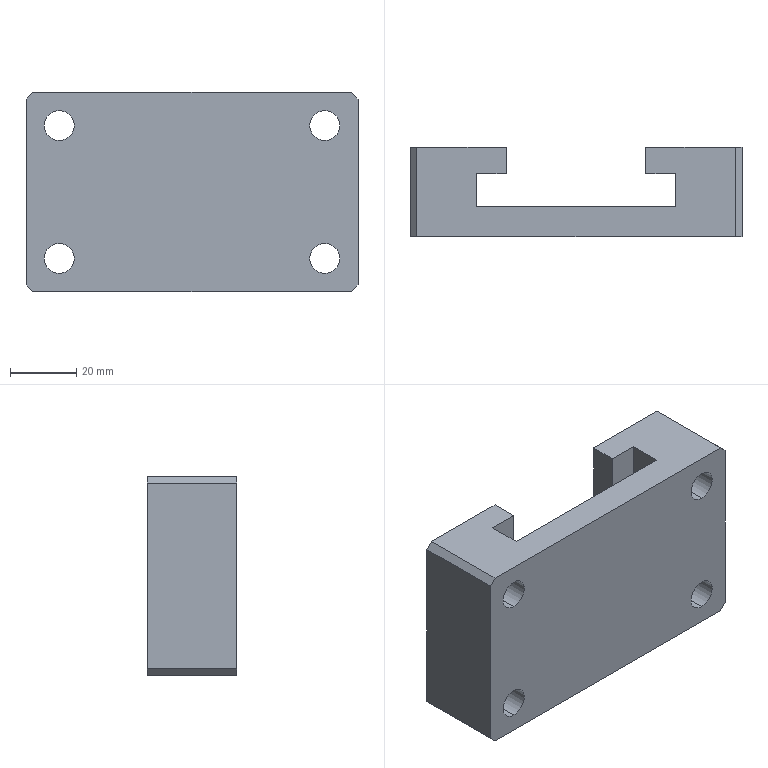Part | SolidWorks | features BaseBody 1 | 1 solid | 38 faces | box 100 x 27 x 60 mm | volume 94682 mm3 | plane 22 | cylinder 16 | commonest cylinder face diameters 9 x8 15 x8
STEP:
#1=CARTESIAN_POINT('',(-40.,4.036,2.5));
#2=VERTEX_POINT('',#1);
#3=CARTESIAN_POINT('',(-40.,4.036,17.5));
#4=VERTEX_POINT('',#3);
#5=CARTESIAN_POINT('',(-40.,4.036,10.));
#6=DIRECTION('',(0.,1.,0.));
#7=DIRECTION('',(0.,0.,1.));
#8=AXIS2_PLACEMENT_3D('',#5,#6,#7);
#9=CIRCLE('',#8,7.5);
#10=EDGE_CURVE('',#2,#4,#9,.T.);
#11=ORIENTED_EDGE('',*,*,#10,.F.);
#12=CARTESIAN_POINT('',(-40.,13.036,2.5));
#13=VERTEX_POINT('',#12);
#14=CARTESIAN_POINT('',(-40.,13.036,2.5));
#15=DIRECTION('',(0.,1.,0.));
#16=VECTOR('',#15,1000.);
#17=LINE('',#14,#16);
#18=EDGE_CURVE('',#2,#13,#17,.T.);
#19=ORIENTED_EDGE('',*,*,#18,.T.);
#20=CARTESIAN_POINT('',(-40.,13.036,17.5));
#21=VERTEX_POINT('',#20);
#22=CARTESIAN_POINT('',(-40.,13.036,10.));
#23=DIRECTION('',(0.,1.,0.));
#24=DIRECTION('',(0.,0.,1.));
#25=AXIS2_PLACEMENT_3D('',#22,#23,#24);
#26=CIRCLE('',#25,7.5);
#27=EDGE_CURVE('',#13,#21,#26,.T.);
#28=ORIENTED_EDGE('',*,*,#27,.T.);
#29=CARTESIAN_POINT('',(-40.,13.036,17.5));
#30=DIRECTION('',(0.,1.,0.));
#31=VECTOR('',#30,1000.);
#32=LINE('',#29,#31);
#33=EDGE_CURVE('',#4,#21,#32,.T.);
#34=ORIENTED_EDGE('',*,*,#33,.F.);
#35=EDGE_LOOP('',(#11,#19,#28,#34));
#36=FACE_OUTER_BOUND('',#35,.T.);
#37=CARTESIAN_POINT('',(-40.,13.036,10.));
#38=DIRECTION('',(0.,1.,0.));
#39=DIRECTION('',(0.,0.,1.));
#40=AXIS2_PLACEMENT_3D('',#37,#38,#39);
#41=CYLINDRICAL_SURFACE('',#40,7.5);
#42=ADVANCED_FACE('',(#36),#41,.F.);
#43=CARTESIAN_POINT('',(-40.,-13.964,5.5));
#44=VERTEX_POINT('',#43);
#45=CARTESIAN_POINT('',(-40.,-13.964,14.5));
#46=VERTEX_POINT('',#45);
#47=CARTESIAN_POINT('',(-40.,-13.964,10.));
#48=DIRECTION('',(0.,1.,0.));
#49=DIRECTION('',(0.,0.,1.));
#50=AXIS2_PLACEMENT_3D('',#47,#48,#49);
#51=CIRCLE('',#50,4.5);
#52=EDGE_CURVE('',#44,#46,#51,.T.);
#53=ORIENTED_EDGE('',*,*,#52,.F.);
#54=CARTESIAN_POINT('',(-40.,4.036,5.5));
#55=VERTEX_POINT('',#54);
#56=CARTESIAN_POINT('',(-40.,13.036,5.5));
#57=DIRECTION('',(0.,1.,0.));
#58=VECTOR('',#57,1000.);
#59=LINE('',#56,#58);
#60=EDGE_CURVE('',#44,#55,#59,.T.);
#61=ORIENTED_EDGE('',*,*,#60,.T.);
#62=CARTESIAN_POINT('',(-40.,4.036,14.5));
#63=VERTEX_POINT('',#62);
#64=CARTESIAN_POINT('',(-40.,4.036,10.));
#65=DIRECTION('',(0.,1.,0.));
#66=DIRECTION('',(0.,0.,1.));
#67=AXIS2_PLACEMENT_3D('',#64,#65,#66);
#68=CIRCLE('',#67,4.5);
#69=EDGE_CURVE('',#55,#63,#68,.T.);
#70=ORIENTED_EDGE('',*,*,#69,.T.);
#71=CARTESIAN_POINT('',(-40.,13.036,14.5));
#72=DIRECTION('',(0.,1.,0.));
#73=VECTOR('',#72,1000.);
#74=LINE('',#71,#73);
#75=EDGE_CURVE('',#46,#63,#74,.T.);
#76=ORIENTED_EDGE('',*,*,#75,.F.);
#77=EDGE_LOOP('',(#53,#61,#70,#76));
#78=FACE_OUTER_BOUND('',#77,.T.);
#79=CARTESIAN_POINT('',(-40.,13.036,10.));
#80=DIRECTION('',(0.,1.,0.));
#81=DIRECTION('',(0.,0.,1.));
#82=AXIS2_PLACEMENT_3D('',#79,#80,#81);
#83=CYLINDRICAL_SURFACE('',#82,4.5);
#84=ADVANCED_FACE('',(#78),#83,.F.);
#85=CARTESIAN_POINT('',(40.,4.036,42.5));
#86=VERTEX_POINT('',#85);
#87=CARTESIAN_POINT('',(40.,4.036,57.5));
#88=VERTEX_POINT('',#87);
#89=CARTESIAN_POINT('',(40.,4.036,50.));
#90=DIRECTION('',(0.,1.,0.));
#91=DIRECTION('',(0.,0.,1.));
#92=AXIS2_PLACEMENT_3D('',#89,#90,#91);
#93=CIRCLE('',#92,7.5);
#94=EDGE_CURVE('',#86,#88,#93,.T.);
#95=ORIENTED_EDGE('',*,*,#94,.F.);
#96=CARTESIAN_POINT('',(40.,13.036,42.5));
#97=VERTEX_POINT('',#96);
#98=CARTESIAN_POINT('',(40.,13.036,42.5));
#99=DIRECTION('',(0.,1.,0.));
#100=VECTOR('',#99,1000.);
#101=LINE('',#98,#100);
#102=EDGE_CURVE('',#86,#97,#101,.T.);
#103=ORIENTED_EDGE('',*,*,#102,.T.);
#104=CARTESIAN_POINT('',(40.,13.036,57.5));
#105=VERTEX_POINT('',#104);
#106=CARTESIAN_POINT('',(40.,13.036,50.));
#107=DIRECTION('',(0.,1.,0.));
#108=DIRECTION('',(0.,0.,1.));
#109=AXIS2_PLACEMENT_3D('',#106,#107,#108);
#110=CIRCLE('',#109,7.5);
#111=EDGE_CURVE('',#97,#105,#110,.T.);
#112=ORIENTED_EDGE('',*,*,#111,.T.);
#113=CARTESIAN_POINT('',(40.,13.036,57.5));
#114=DIRECTION('',(0.,1.,0.));
#115=VECTOR('',#114,1000.);
#116=LINE('',#113,#115);
#117=EDGE_CURVE('',#88,#105,#116,.T.);
#118=ORIENTED_EDGE('',*,*,#117,.F.);
#119=EDGE_LOOP('',(#95,#103,#112,#118));
#120=FACE_OUTER_BOUND('',#119,.T.);
#121=CARTESIAN_POINT('',(40.,13.036,50.));
#122=DIRECTION('',(0.,1.,0.));
#123=DIRECTION('',(0.,0.,1.));
#124=AXIS2_PLACEMENT_3D('',#121,#122,#123);
#125=CYLINDRICAL_SURFACE('',#124,7.5);
#126=ADVANCED_FACE('',(#120),#125,.F.);
#127=CARTESIAN_POINT('',(40.,-13.964,45.5));
#128=VERTEX_POINT('',#127);
#129=CARTESIAN_POINT('',(40.,-13.964,54.5));
#130=VERTEX_POINT('',#129);
#131=CARTESIAN_POINT('',(40.,-13.964,50.));
#132=DIRECTION('',(0.,1.,0.));
#133=DIRECTION('',(0.,0.,1.));
#134=AXIS2_PLACEMENT_3D('',#131,#132,#133);
#135=CIRCLE('',#134,4.5);
#136=EDGE_CURVE('',#128,#130,#135,.T.);
#137=ORIENTED_EDGE('',*,*,#136,.F.);
#138=CARTESIAN_POINT('',(40.,4.036,45.5));
#139=VERTEX_POINT('',#138);
#140=CARTESIAN_POINT('',(40.,13.036,45.5));
#141=DIRECTION('',(0.,1.,0.));
#142=VECTOR('',#141,1000.);
#143=LINE('',#140,#142);
#144=EDGE_CURVE('',#128,#139,#143,.T.);
#145=ORIENTED_EDGE('',*,*,#144,.T.);
#146=CARTESIAN_POINT('',(40.,4.036,54.5));
#147=VERTEX_POINT('',#146);
#148=CARTESIAN_POINT('',(40.,4.036,50.));
#149=DIRECTION('',(0.,1.,0.));
#150=DIRECTION('',(0.,0.,1.));
#151=AXIS2_PLACEMENT_3D('',#148,#149,#150);
#152=CIRCLE('',#151,4.5);
#153=EDGE_CURVE('',#139,#147,#152,.T.);
#154=ORIENTED_EDGE('',*,*,#153,.T.);
#155=CARTESIAN_POINT('',(40.,13.036,54.5));
#156=DIRECTION('',(0.,1.,0.));
#157=VECTOR('',#156,1000.);
#158=LINE('',#155,#157);
#159=EDGE_CURVE('',#130,#147,#158,.T.);
#160=ORIENTED_EDGE('',*,*,#159,.F.);
#161=EDGE_LOOP('',(#137,#145,#154,#160));
#162=FACE_OUTER_BOUND('',#161,.T.);
#163=CARTESIAN_POINT('',(40.,13.036,50.));
#164=DIRECTION('',(0.,1.,0.));
#165=DIRECTION('',(0.,0.,1.));
#166=AXIS2_PLACEMENT_3D('',#163,#164,#165);
#167=CYLINDRICAL_SURFACE('',#166,4.5);
#168=ADVANCED_FACE('',(#162),#167,.F.);
#169=CARTESIAN_POINT('',(-40.,4.036,42.5));
#170=VERTEX_POINT('',#169);
#171=CARTESIAN_POINT('',(-40.,4.036,57.5));
#172=VERTEX_POINT('',#171);
#173=CARTESIAN_POINT('',(-40.,4.036,50.));
#174=DIRECTION('',(0.,1.,0.));
#175=DIRECTION('',(0.,0.,1.));
#176=AXIS2_PLACEMENT_3D('',#173,#174,#175);
#177=CIRCLE('',#176,7.5);
#178=EDGE_CURVE('',#170,#172,#177,.T.);
#179=ORIENTED_EDGE('',*,*,#178,.F.);
#180=CARTESIAN_POINT('',(-40.,13.036,42.5));
#181=VERTEX_POINT('',#180);
#182=CARTESIAN_POINT('',(-40.,13.036,42.5));
#183=DIRECTION('',(0.,1.,0.));
#184=VECTOR('',#183,1000.);
#185=LINE('',#182,#184);
#186=EDGE_CURVE('',#170,#181,#185,.T.);
#187=ORIENTED_EDGE('',*,*,#186,.T.);
#188=CARTESIAN_POINT('',(-40.,13.036,57.5));
#189=VERTEX_POINT('',#188);
#190=CARTESIAN_POINT('',(-40.,13.036,50.));
#191=DIRECTION('',(0.,1.,0.));
#192=DIRECTION('',(0.,0.,1.));
#193=AXIS2_PLACEMENT_3D('',#190,#191,#192);
#194=CIRCLE('',#193,7.5);
#195=EDGE_CURVE('',#181,#189,#194,.T.);
#196=ORIENTED_EDGE('',*,*,#195,.T.);
#197=CARTESIAN_POINT('',(-40.,13.036,57.5));
#198=DIRECTION('',(0.,1.,0.));
#199=VECTOR('',#198,1000.);
#200=LINE('',#197,#199);
#201=EDGE_CURVE('',#172,#189,#200,.T.);
#202=ORIENTED_EDGE('',*,*,#201,.F.);
#203=EDGE_LOOP('',(#179,#187,#196,#202));
#204=FACE_OUTER_BOUND('',#203,.T.);
#205=CARTESIAN_POINT('',(-40.,13.036,50.));
#206=DIRECTION('',(0.,1.,0.));
#207=DIRECTION('',(0.,0.,1.));
#208=AXIS2_PLACEMENT_3D('',#205,#206,#207);
#209=CYLINDRICAL_SURFACE('',#208,7.5);
#210=ADVANCED_FACE('',(#204),#209,.F.);
#211=CARTESIAN_POINT('',(-40.,-13.964,45.5));
#212=VERTEX_POINT('',#211);
#213=CARTESIAN_POINT('',(-40.,-13.964,54.5));
#214=VERTEX_POINT('',#213);
#215=CARTESIAN_POINT('',(-40.,-13.964,50.));
#216=DIRECTION('',(0.,1.,0.));
#217=DIRECTION('',(0.,0.,1.));
#218=AXIS2_PLACEMENT_3D('',#215,#216,#217);
#219=CIRCLE('',#218,4.5);
#220=EDGE_CURVE('',#212,#214,#219,.T.);
#221=ORIENTED_EDGE('',*,*,#220,.F.);
#222=CARTESIAN_POINT('',(-40.,4.036,45.5));
#223=VERTEX_POINT('',#222);
#224=CARTESIAN_POINT('',(-40.,13.036,45.5));
#225=DIRECTION('',(0.,1.,0.));
#226=VECTOR('',#225,1000.);
#227=LINE('',#224,#226);
#228=EDGE_CURVE('',#212,#223,#227,.T.);
#229=ORIENTED_EDGE('',*,*,#228,.T.);
#230=CARTESIAN_POINT('',(-40.,4.036,54.5));
#231=VERTEX_POINT('',#230);
#232=CARTESIAN_POINT('',(-40.,4.036,50.));
#233=DIRECTION('',(0.,1.,0.));
#234=DIRECTION('',(0.,0.,1.));
#235=AXIS2_PLACEMENT_3D('',#232,#233,#234);
#236=CIRCLE('',#235,4.5);
#237=EDGE_CURVE('',#223,#231,#236,.T.);
#238=ORIENTED_EDGE('',*,*,#237,.T.);
#239=CARTESIAN_POINT('',(-40.,13.036,54.5));
#240=DIRECTION('',(0.,1.,0.));
#241=VECTOR('',#240,1000.);
#242=LINE('',#239,#241);
#243=EDGE_CURVE('',#214,#231,#242,.T.);
#244=ORIENTED_EDGE('',*,*,#243,.F.);
#245=EDGE_LOOP('',(#221,#229,#238,#244));
#246=FACE_OUTER_BOUND('',#245,.T.);
#247=CARTESIAN_POINT('',(-40.,13.036,50.));
#248=DIRECTION('',(0.,1.,0.));
#249=DIRECTION('',(0.,0.,1.));
#250=AXIS2_PLACEMENT_3D('',#247,#248,#249);
#251=CYLINDRICAL_SURFACE('',#250,4.5);
#252=ADVANCED_FACE('',(#246),#251,.F.);
#253=CARTESIAN_POINT('',(40.,4.036,2.5));
#254=VERTEX_POINT('',#253);
#255=CARTESIAN_POINT('',(40.,4.036,17.5));
#256=VERTEX_POINT('',#255);
#257=CARTESIAN_POINT('',(40.,4.036,10.));
#258=DIRECTION('',(0.,1.,0.));
#259=DIRECTION('',(0.,0.,1.));
#260=AXIS2_PLACEMENT_3D('',#257,#258,#259);
#261=CIRCLE('',#260,7.5);
#262=EDGE_CURVE('',#254,#256,#261,.T.);
#263=ORIENTED_EDGE('',*,*,#262,.F.);
#264=CARTESIAN_POINT('',(40.,13.036,2.5));
#265=VERTEX_POINT('',#264);
#266=CARTESIAN_POINT('',(40.,13.036,2.5));
#267=DIRECTION('',(0.,1.,0.));
#268=VECTOR('',#267,1000.);
#269=LINE('',#266,#268);
#270=EDGE_CURVE('',#254,#265,#269,.T.);
#271=ORIENTED_EDGE('',*,*,#270,.T.);
#272=CARTESIAN_POINT('',(40.,13.036,17.5));
#273=VERTEX_POINT('',#272);
#274=CARTESIAN_POINT('',(40.,13.036,10.));
#275=DIRECTION('',(0.,1.,0.));
#276=DIRECTION('',(0.,0.,1.));
#277=AXIS2_PLACEMENT_3D('',#274,#275,#276);
#278=CIRCLE('',#277,7.5);
#279=EDGE_CURVE('',#265,#273,#278,.T.);
#280=ORIENTED_EDGE('',*,*,#279,.T.);
#281=CARTESIAN_POINT('',(40.,13.036,17.5));
#282=DIRECTION('',(0.,1.,0.));
#283=VECTOR('',#282,1000.);
#284=LINE('',#281,#283);
#285=EDGE_CURVE('',#256,#273,#284,.T.);
#286=ORIENTED_EDGE('',*,*,#285,.F.);
#287=EDGE_LOOP('',(#263,#271,#280,#286));
#288=FACE_OUTER_BOUND('',#287,.T.);
#289=CARTESIAN_POINT('',(40.,13.036,10.));
#290=DIRECTION('',(0.,1.,0.));
#291=DIRECTION('',(0.,0.,1.));
#292=AXIS2_PLACEMENT_3D('',#289,#290,#291);
#293=CYLINDRICAL_SURFACE('',#292,7.5);
#294=ADVANCED_FACE('',(#288),#293,.F.);
#295=CARTESIAN_POINT('',(40.,-13.964,5.5));
#296=VERTEX_POINT('',#295);
#297=CARTESIAN_POINT('',(40.,-13.964,14.5));
#298=VERTEX_POINT('',#297);
#299=CARTESIAN_POINT('',(40.,-13.964,10.));
#300=DIRECTION('',(0.,1.,0.));
#301=DIRECTION('',(0.,0.,1.));
#302=AXIS2_PLACEMENT_3D('',#299,#300,#301);
#303=CIRCLE('',#302,4.5);
#304=EDGE_CURVE('',#296,#298,#303,.T.);
#305=ORIENTED_EDGE('',*,*,#304,.F.);
#306=CARTESIAN_POINT('',(40.,4.036,5.5));
#307=VERTEX_POINT('',#306);
#308=CARTESIAN_POINT('',(40.,13.036,5.5));
#309=DIRECTION('',(0.,1.,0.));
#310=VECTOR('',#309,1000.);
#311=LINE('',#308,#310);
#312=EDGE_CURVE('',#296,#307,#311,.T.);
#313=ORIENTED_EDGE('',*,*,#312,.T.);
#314=CARTESIAN_POINT('',(40.,4.036,14.5));
#315=VERTEX_POINT('',#314);
#316=CARTESIAN_POINT('',(40.,4.036,10.));
#317=DIRECTION('',(0.,1.,0.));
#318=DIRECTION('',(0.,0.,1.));
#319=AXIS2_PLACEMENT_3D('',#316,#317,#318);
#320=CIRCLE('',#319,4.5);
#321=EDGE_CURVE('',#307,#315,#320,.T.);
#322=ORIENTED_EDGE('',*,*,#321,.T.);
#323=CARTESIAN_POINT('',(40.,13.036,14.5));
#324=DIRECTION('',(0.,1.,0.));
#325=VECTOR('',#324,1000.);
#326=LINE('',#323,#325);
#327=EDGE_CURVE('',#298,#315,#326,.T.);
#328=ORIENTED_EDGE('',*,*,#327,.F.);
#329=EDGE_LOOP('',(#305,#313,#322,#328));
#330=FACE_OUTER_BOUND('',#329,.T.);
#331=CARTESIAN_POINT('',(40.,13.036,10.));
#332=DIRECTION('',(0.,1.,0.));
#333=DIRECTION('',(0.,0.,1.));
#334=AXIS2_PLACEMENT_3D('',#331,#332,#333);
#335=CYLINDRICAL_SURFACE('',#334,4.5);
#336=ADVANCED_FACE('',(#330),#335,.F.);
#337=CARTESIAN_POINT('',(30.,5.036,0.));
#338=VERTEX_POINT('',#337);
#339=CARTESIAN_POINT('',(30.,-4.964,0.));
#340=VERTEX_POINT('',#339);
#341=CARTESIAN_POINT('',(30.,5.036,0.));
#342=DIRECTION('',(0.,-1.,0.));
#343=VECTOR('',#342,1000.);
#344=LINE('',#341,#343);
#345=EDGE_CURVE('',#338,#340,#344,.T.);
#346=ORIENTED_EDGE('',*,*,#345,.T.);
#347=CARTESIAN_POINT('',(30.,-4.964,60.));
#348=VERTEX_POINT('',#347);
#349=CARTESIAN_POINT('',(30.,-4.964,60.));
#350=DIRECTION('',(0.,0.,-1.));
#351=VECTOR('',#350,1000.);
#352=LINE('',#349,#351);
#353=EDGE_CURVE('',#348,#340,#352,.T.);
#354=ORIENTED_EDGE('',*,*,#353,.F.);
#355=CARTESIAN_POINT('',(30.,5.036,60.));
#356=VERTEX_POINT('',#355);
#357=CARTESIAN_POINT('',(30.,5.036,60.));
#358=DIRECTION('',(0.,-1.,0.));
#359=VECTOR('',#358,1000.);
#360=LINE('',#357,#359);
#361=EDGE_CURVE('',#356,#348,#360,.T.);
#362=ORIENTED_EDGE('',*,*,#361,.F.);
#363=CARTESIAN_POINT('',(30.,5.036,60.));
#364=DIRECTION('',(0.,0.,-1.));
#365=VECTOR('',#364,1000.);
#366=LINE('',#363,#365);
#367=EDGE_CURVE('',#356,#338,#366,.T.);
#368=ORIENTED_EDGE('',*,*,#367,.T.);
#369=EDGE_LOOP('',(#346,#354,#362,#368));
#370=FACE_OUTER_BOUND('',#369,.T.);
#371=CARTESIAN_POINT('',(30.,5.036,60.));
#372=DIRECTION('',(1.,0.,0.));
#373=DIRECTION('',(0.,0.,-1.));
#374=AXIS2_PLACEMENT_3D('',#371,#372,#373);
#375=PLANE('',#374);
#376=ADVANCED_FACE('',(#370),#375,.F.);
#377=CARTESIAN_POINT('',(-30.,-4.964,0.));
#378=VERTEX_POINT('',#377);
#379=CARTESIAN_POINT('',(-30.,-4.964,0.));
#380=DIRECTION('',(-1.,0.,0.));
#381=VECTOR('',#380,1000.);
#382=LINE('',#379,#381);
#383=EDGE_CURVE('',#340,#378,#382,.T.);
#384=ORIENTED_EDGE('',*,*,#383,.T.);
#385=CARTESIAN_POINT('',(-30.,-4.964,60.));
#386=VERTEX_POINT('',#385);
#387=CARTESIAN_POINT('',(-30.,-4.964,60.));
#388=DIRECTION('',(0.,0.,-1.));
#389=VECTOR('',#388,1000.);
#390=LINE('',#387,#389);
#391=EDGE_CURVE('',#386,#378,#390,.T.);
#392=ORIENTED_EDGE('',*,*,#391,.F.);
#393=CARTESIAN_POINT('',(-30.,-4.964,60.));
#394=DIRECTION('',(-1.,0.,0.));
#395=VECTOR('',#394,1000.);
#396=LINE('',#393,#395);
#397=EDGE_CURVE('',#348,#386,#396,.T.);
#398=ORIENTED_EDGE('',*,*,#397,.F.);
#399=ORIENTED_EDGE('',*,*,#353,.T.);
#400=EDGE_LOOP('',(#384,#392,#398,#399));
#401=FACE_OUTER_BOUND('',#400,.T.);
#402=CARTESIAN_POINT('',(-30.,-4.964,60.));
#403=DIRECTION('',(0.,-1.,0.));
#404=DIRECTION('',(0.,0.,-1.));
#405=AXIS2_PLACEMENT_3D('',#402,#403,#404);
#406=PLANE('',#405);
#407=ADVANCED_FACE('',(#401),#406,.F.);
#408=CARTESIAN_POINT('',(-30.,5.036,0.));
#409=VERTEX_POINT('',#408);
#410=CARTESIAN_POINT('',(-30.,5.036,0.));
#411=DIRECTION('',(0.,1.,0.));
#412=VECTOR('',#411,1000.);
#413=LINE('',#410,#412);
#414=EDGE_CURVE('',#378,#409,#413,.T.);
#415=ORIENTED_EDGE('',*,*,#414,.T.);
#416=CARTESIAN_POINT('',(-30.,5.036,60.));
#417=VERTEX_POINT('',#416);
#418=CARTESIAN_POINT('',(-30.,5.036,60.));
#419=DIRECTION('',(0.,0.,-1.));
#420=VECTOR('',#419,1000.);
#421=LINE('',#418,#420);
#422=EDGE_CURVE('',#417,#409,#421,.T.);
#423=ORIENTED_EDGE('',*,*,#422,.F.);
#424=CARTESIAN_POINT('',(-30.,5.036,60.));
#425=DIRECTION('',(0.,1.,0.));
#426=VECTOR('',#425,1000.);
#427=LINE('',#424,#426);
#428=EDGE_CURVE('',#386,#417,#427,.T.);
#429=ORIENTED_EDGE('',*,*,#428,.F.);
#430=ORIENTED_EDGE('',*,*,#391,.T.);
#431=EDGE_LOOP('',(#415,#423,#429,#430));
#432=FACE_OUTER_BOUND('',#431,.T.);
#433=CARTESIAN_POINT('',(-30.,5.036,60.));
#434=DIRECTION('',(-1.,0.,0.));
#435=DIRECTION('',(0.,0.,1.));
#436=AXIS2_PLACEMENT_3D('',#433,#434,#435);
#437=PLANE('',#436);
#438=ADVANCED_FACE('',(#432),#437,.F.);
#439=CARTESIAN_POINT('',(-21.,5.036,0.));
#440=VERTEX_POINT('',#439);
#441=CARTESIAN_POINT('',(-30.,5.036,0.));
#442=DIRECTION('',(1.,0.,0.));
#443=VECTOR('',#442,1000.);
#444=LINE('',#441,#443);
#445=EDGE_CURVE('',#409,#440,#444,.T.);
#446=ORIENTED_EDGE('',*,*,#445,.T.);
#447=CARTESIAN_POINT('',(-21.,5.036,60.));
#448=VERTEX_POINT('',#447);
#449=CARTESIAN_POINT('',(-21.,5.036,60.));
#450=DIRECTION('',(0.,0.,-1.));
#451=VECTOR('',#450,1000.);
#452=LINE('',#449,#451);
#453=EDGE_CURVE('',#448,#440,#452,.T.);
#454=ORIENTED_EDGE('',*,*,#453,.F.);
#455=CARTESIAN_POINT('',(-30.,5.036,60.));
#456=DIRECTION('',(1.,0.,0.));
#457=VECTOR('',#456,1000.);
#458=LINE('',#455,#457);
#459=EDGE_CURVE('',#417,#448,#458,.T.);
#460=ORIENTED_EDGE('',*,*,#459,.F.);
#461=ORIENTED_EDGE('',*,*,#422,.T.);
#462=EDGE_LOOP('',(#446,#454,#460,#461));
#463=FACE_OUTER_BOUND('',#462,.T.);
#464=CARTESIAN_POINT('',(-30.,5.036,60.));
#465=DIRECTION('',(0.,1.,0.));
#466=DIRECTION('',(-1.,0.,0.));
#467=AXIS2_PLACEMENT_3D('',#464,#465,#466);
#468=PLANE('',#467);
#469=ADVANCED_FACE('',(#463),#468,.F.);
#470=CARTESIAN_POINT('',(-21.,13.036,0.));
#471=VERTEX_POINT('',#470);
#472=CARTESIAN_POINT('',(-21.,13.036,0.));
#473=DIRECTION('',(0.,1.,0.));
#474=VECTOR('',#473,1000.);
#475=LINE('',#472,#474);
#476=EDGE_CURVE('',#440,#471,#475,.T.);
#477=ORIENTED_EDGE('',*,*,#476,.T.);
#478=CARTESIAN_POINT('',(-21.,13.036,60.));
#479=VERTEX_POINT('',#478);
#480=CARTESIAN_POINT('',(-21.,13.036,60.));
#481=DIRECTION('',(0.,0.,-1.));
#482=VECTOR('',#481,1000.);
#483=LINE('',#480,#482);
#484=EDGE_CURVE('',#479,#471,#483,.T.);
#485=ORIENTED_EDGE('',*,*,#484,.F.);
#486=CARTESIAN_POINT('',(-21.,13.036,60.));
#487=DIRECTION('',(0.,1.,0.));
#488=VECTOR('',#487,1000.);
#489=LINE('',#486,#488);
#490=EDGE_CURVE('',#448,#479,#489,.T.);
#491=ORIENTED_EDGE('',*,*,#490,.F.);
#492=ORIENTED_EDGE('',*,*,#453,.T.);
#493=EDGE_LOOP('',(#477,#485,#491,#492));
#494=FACE_OUTER_BOUND('',#493,.T.);
#495=CARTESIAN_POINT('',(-21.,13.036,60.));
#496=DIRECTION('',(-1.,0.,0.));
#497=DIRECTION('',(0.,0.,1.));
#498=AXIS2_PLACEMENT_3D('',#495,#496,#497);
#499=PLANE('',#498);
#500=ADVANCED_FACE('',(#494),#499,.F.);
#501=CARTESIAN_POINT('',(-40.,13.036,10.));
#502=DIRECTION('',(0.,1.,0.));
#503=DIRECTION('',(0.,0.,1.));
#504=AXIS2_PLACEMENT_3D('',#501,#502,#503);
#505=CIRCLE('',#504,7.5);
#506=EDGE_CURVE('',#21,#13,#505,.T.);
#507=ORIENTED_EDGE('',*,*,#506,.F.);
#508=ORIENTED_EDGE('',*,*,#27,.F.);
#509=EDGE_LOOP('',(#507,#508));
#510=FACE_BOUND('',#509,.T.);
#511=CARTESIAN_POINT('',(-40.,13.036,50.));
#512=DIRECTION('',(0.,1.,0.));
#513=DIRECTION('',(0.,0.,1.));
#514=AXIS2_PLACEMENT_3D('',#511,#512,#513);
#515=CIRCLE('',#514,7.5);
#516=EDGE_CURVE('',#189,#181,#515,.T.);
#517=ORIENTED_EDGE('',*,*,#516,.F.);
#518=ORIENTED_EDGE('',*,*,#195,.F.);
#519=EDGE_LOOP('',(#517,#518));
#520=FACE_BOUND('',#519,.T.);
#521=CARTESIAN_POINT('',(-48.,13.036,0.));
#522=VERTEX_POINT('',#521);
#523=CARTESIAN_POINT('',(-50.,13.036,0.));
#524=DIRECTION('',(-1.,0.,0.));
#525=VECTOR('',#524,1000.);
#526=LINE('',#523,#525);
#527=EDGE_CURVE('',#471,#522,#526,.T.);
#528=ORIENTED_EDGE('',*,*,#527,.T.);
#529=CARTESIAN_POINT('',(-50.,13.036,2.));
#530=VERTEX_POINT('',#529);
#531=CARTESIAN_POINT('',(-50.,13.036,2.));
#532=DIRECTION('',(-0.7071,0.,0.7071));
#533=VECTOR('',#532,1000.);
#534=LINE('',#531,#533);
#535=EDGE_CURVE('',#522,#530,#534,.T.);
#536=ORIENTED_EDGE('',*,*,#535,.T.);
#537=CARTESIAN_POINT('',(-50.,13.036,58.));
#538=VERTEX_POINT('',#537);
#539=CARTESIAN_POINT('',(-50.,13.036,60.));
#540=DIRECTION('',(0.,0.,-1.));
#541=VECTOR('',#540,1000.);
#542=LINE('',#539,#541);
#543=EDGE_CURVE('',#538,#530,#542,.T.);
#544=ORIENTED_EDGE('',*,*,#543,.F.);
#545=CARTESIAN_POINT('',(-48.,13.036,60.));
#546=VERTEX_POINT('',#545);
#547=CARTESIAN_POINT('',(-48.,13.036,60.));
#548=DIRECTION('',(0.7071,0.,0.7071));
#549=VECTOR('',#548,1000.);
#550=LINE('',#547,#549);
#551=EDGE_CURVE('',#538,#546,#550,.T.);
#552=ORIENTED_EDGE('',*,*,#551,.T.);
#553=CARTESIAN_POINT('',(-50.,13.036,60.));
#554=DIRECTION('',(-1.,0.,0.));
#555=VECTOR('',#554,1000.);
#556=LINE('',#553,#555);
#557=EDGE_CURVE('',#479,#546,#556,.T.);
#558=ORIENTED_EDGE('',*,*,#557,.F.);
#559=ORIENTED_EDGE('',*,*,#484,.T.);
#560=EDGE_LOOP('',(#528,#536,#544,#552,#558,#559));
#561=FACE_OUTER_BOUND('',#560,.T.);
#562=CARTESIAN_POINT('',(-50.,13.036,60.));
#563=DIRECTION('',(0.,-1.,0.));
#564=DIRECTION('',(1.,0.,0.));
#565=AXIS2_PLACEMENT_3D('',#562,#563,#564);
#566=PLANE('',#565);
#567=ADVANCED_FACE('',(#510,#520,#561),#566,.F.);
#568=ORIENTED_EDGE('',*,*,#543,.T.);
#569=CARTESIAN_POINT('',(-50.,-13.964,2.));
#570=VERTEX_POINT('',#569);
#571=CARTESIAN_POINT('',(-50.,-10.964,2.));
#572=DIRECTION('',(0.,-1.,0.));
#573=VECTOR('',#572,1000.);
#574=LINE('',#571,#573);
#575=EDGE_CURVE('',#530,#570,#574,.T.);
#576=ORIENTED_EDGE('',*,*,#575,.T.);
#577=CARTESIAN_POINT('',(-50.,-13.964,58.));
#578=VERTEX_POINT('',#577);
#579=CARTESIAN_POINT('',(-50.,-13.964,60.));
#580=DIRECTION('',(0.,0.,-1.));
#581=VECTOR('',#580,1000.);
#582=LINE('',#579,#581);
#583=EDGE_CURVE('',#578,#570,#582,.T.);
#584=ORIENTED_EDGE('',*,*,#583,.F.);
#585=CARTESIAN_POINT('',(-50.,13.036,58.));
#586=DIRECTION('',(0.,1.,0.));
#587=VECTOR('',#586,1000.);
#588=LINE('',#585,#587);
#589=EDGE_CURVE('',#578,#538,#588,.T.);
#590=ORIENTED_EDGE('',*,*,#589,.T.);
#591=EDGE_LOOP('',(#568,#576,#584,#590));
#592=FACE_OUTER_BOUND('',#591,.T.);
#593=CARTESIAN_POINT('',(-50.,-10.964,60.));
#594=DIRECTION('',(1.,0.,0.));
#595=DIRECTION('',(0.,0.,-1.));
#596=AXIS2_PLACEMENT_3D('',#593,#594,#595);
#597=PLANE('',#596);
#598=ADVANCED_FACE('',(#592),#597,.F.);
#599=CARTESIAN_POINT('',(-40.,-13.964,10.));
#600=DIRECTION('',(0.,1.,0.));
#601=DIRECTION('',(0.,0.,1.));
#602=AXIS2_PLACEMENT_3D('',#599,#600,#601);
#603=CIRCLE('',#602,4.5);
#604=EDGE_CURVE('',#46,#44,#603,.T.);
#605=ORIENTED_EDGE('',*,*,#604,.T.);
#606=ORIENTED_EDGE('',*,*,#52,.T.);
#607=EDGE_LOOP('',(#605,#606));
#608=FACE_BOUND('',#607,.T.);
#609=CARTESIAN_POINT('',(40.,-13.964,50.));
#610=DIRECTION('',(0.,1.,0.));
#611=DIRECTION('',(0.,0.,1.));
#612=AXIS2_PLACEMENT_3D('',#609,#610,#611);
#613=CIRCLE('',#612,4.5);
#614=EDGE_CURVE('',#130,#128,#613,.T.);
#615=ORIENTED_EDGE('',*,*,#614,.T.);
#616=ORIENTED_EDGE('',*,*,#136,.T.);
#617=EDGE_LOOP('',(#615,#616));
#618=FACE_BOUND('',#617,.T.);
#619=CARTESIAN_POINT('',(-40.,-13.964,50.));
#620=DIRECTION('',(0.,1.,0.));
#621=DIRECTION('',(0.,0.,1.));
#622=AXIS2_PLACEMENT_3D('',#619,#620,#621);
#623=CIRCLE('',#622,4.5);
#624=EDGE_CURVE('',#214,#212,#623,.T.);
#625=ORIENTED_EDGE('',*,*,#624,.T.);
#626=ORIENTED_EDGE('',*,*,#220,.T.);
#627=EDGE_LOOP('',(#625,#626));
#628=FACE_BOUND('',#627,.T.);
#629=CARTESIAN_POINT('',(40.,-13.964,10.));
#630=DIRECTION('',(0.,1.,0.));
#631=DIRECTION('',(0.,0.,1.));
#632=AXIS2_PLACEMENT_3D('',#629,#630,#631);
#633=CIRCLE('',#632,4.5);
#634=EDGE_CURVE('',#298,#296,#633,.T.);
#635=ORIENTED_EDGE('',*,*,#634,.T.);
#636=ORIENTED_EDGE('',*,*,#304,.T.);
#637=EDGE_LOOP('',(#635,#636));
#638=FACE_BOUND('',#637,.T.);
#639=ORIENTED_EDGE('',*,*,#583,.T.);
#640=CARTESIAN_POINT('',(-48.,-13.964,0.));
#641=VERTEX_POINT('',#640);
#642=CARTESIAN_POINT('',(-50.,-13.964,2.));
#643=DIRECTION('',(0.7071,0.,-0.7071));
#644=VECTOR('',#643,1000.);
#645=LINE('',#642,#644);
#646=EDGE_CURVE('',#570,#641,#645,.T.);
#647=ORIENTED_EDGE('',*,*,#646,.T.);
#648=CARTESIAN_POINT('',(48.,-13.964,0.));
#649=VERTEX_POINT('',#648);
#650=CARTESIAN_POINT('',(-50.,-13.964,0.));
#651=DIRECTION('',(1.,0.,0.));
#652=VECTOR('',#651,1000.);
#653=LINE('',#650,#652);
#654=EDGE_CURVE('',#641,#649,#653,.T.);
#655=ORIENTED_EDGE('',*,*,#654,.T.);
#656=CARTESIAN_POINT('',(50.,-13.964,2.));
#657=VERTEX_POINT('',#656);
#658=CARTESIAN_POINT('',(50.,-13.964,2.));
#659=DIRECTION('',(0.7071,0.,0.7071));
#660=VECTOR('',#659,1000.);
#661=LINE('',#658,#660);
#662=EDGE_CURVE('',#649,#657,#661,.T.);
#663=ORIENTED_EDGE('',*,*,#662,.T.);
#664=CARTESIAN_POINT('',(50.,-13.964,58.));
#665=VERTEX_POINT('',#664);
#666=CARTESIAN_POINT('',(50.,-13.964,60.));
#667=DIRECTION('',(0.,0.,-1.));
#668=VECTOR('',#667,1000.);
#669=LINE('',#666,#668);
#670=EDGE_CURVE('',#665,#657,#669,.T.);
#671=ORIENTED_EDGE('',*,*,#670,.F.);
#672=CARTESIAN_POINT('',(48.,-13.964,60.));
#673=VERTEX_POINT('',#672);
#674=CARTESIAN_POINT('',(48.,-13.964,60.));
#675=DIRECTION('',(-0.7071,0.,0.7071));
#676=VECTOR('',#675,1000.);
#677=LINE('',#674,#676);
#678=EDGE_CURVE('',#665,#673,#677,.T.);
#679=ORIENTED_EDGE('',*,*,#678,.T.);
#680=CARTESIAN_POINT('',(-48.,-13.964,60.));
#681=VERTEX_POINT('',#680);
#682=CARTESIAN_POINT('',(-50.,-13.964,60.));
#683=DIRECTION('',(1.,0.,0.));
#684=VECTOR('',#683,1000.);
#685=LINE('',#682,#684);
#686=EDGE_CURVE('',#681,#673,#685,.T.);
#687=ORIENTED_EDGE('',*,*,#686,.F.);
#688=CARTESIAN_POINT('',(-48.,-13.964,60.));
#689=DIRECTION('',(-0.7071,0.,-0.7071));
#690=VECTOR('',#689,1000.);
#691=LINE('',#688,#690);
#692=EDGE_CURVE('',#681,#578,#691,.T.);
#693=ORIENTED_EDGE('',*,*,#692,.T.);
#694=EDGE_LOOP('',(#639,#647,#655,#663,#671,#679,#687,#693));
#695=FACE_OUTER_BOUND('',#694,.T.);
#696=CARTESIAN_POINT('',(-50.,-13.964,60.));
#697=DIRECTION('',(0.,1.,0.));
#698=DIRECTION('',(0.,0.,1.));
#699=AXIS2_PLACEMENT_3D('',#696,#697,#698);
#700=PLANE('',#699);
#701=ADVANCED_FACE('',(#608,#618,#628,#638,#695),#700,.F.);
#702=ORIENTED_EDGE('',*,*,#670,.T.);
#703=CARTESIAN_POINT('',(50.,13.036,2.));
#704=VERTEX_POINT('',#703);
#705=CARTESIAN_POINT('',(50.,13.036,2.));
#706=DIRECTION('',(0.,1.,0.));
#707=VECTOR('',#706,1000.);
#708=LINE('',#705,#707);
#709=EDGE_CURVE('',#657,#704,#708,.T.);
#710=ORIENTED_EDGE('',*,*,#709,.T.);
#711=CARTESIAN_POINT('',(50.,13.036,58.));
#712=VERTEX_POINT('',#711);
#713=CARTESIAN_POINT('',(50.,13.036,60.));
#714=DIRECTION('',(0.,0.,-1.));
#715=VECTOR('',#714,1000.);
#716=LINE('',#713,#715);
#717=EDGE_CURVE('',#712,#704,#716,.T.);
#718=ORIENTED_EDGE('',*,*,#717,.F.);
#719=CARTESIAN_POINT('',(50.,-13.964,58.));
#720=DIRECTION('',(0.,-1.,0.));
#721=VECTOR('',#720,1000.);
#722=LINE('',#719,#721);
#723=EDGE_CURVE('',#712,#665,#722,.T.);
#724=ORIENTED_EDGE('',*,*,#723,.T.);
#725=EDGE_LOOP('',(#702,#710,#718,#724));
#726=FACE_OUTER_BOUND('',#725,.T.);
#727=CARTESIAN_POINT('',(50.,13.036,60.));
#728=DIRECTION('',(-1.,0.,0.));
#729=DIRECTION('',(0.,0.,1.));
#730=AXIS2_PLACEMENT_3D('',#727,#728,#729);
#731=PLANE('',#730);
#732=ADVANCED_FACE('',(#726),#731,.F.);
#733=CARTESIAN_POINT('',(40.,13.036,50.));
#734=DIRECTION('',(0.,1.,0.));
#735=DIRECTION('',(0.,0.,1.));
#736=AXIS2_PLACEMENT_3D('',#733,#734,#735);
#737=CIRCLE('',#736,7.5);
#738=EDGE_CURVE('',#105,#97,#737,.T.);
#739=ORIENTED_EDGE('',*,*,#738,.F.);
#740=ORIENTED_EDGE('',*,*,#111,.F.);
#741=EDGE_LOOP('',(#739,#740));
#742=FACE_BOUND('',#741,.T.);
#743=CARTESIAN_POINT('',(40.,13.036,10.));
#744=DIRECTION('',(0.,1.,0.));
#745=DIRECTION('',(0.,0.,1.));
#746=AXIS2_PLACEMENT_3D('',#743,#744,#745);
#747=CIRCLE('',#746,7.5);
#748=EDGE_CURVE('',#273,#265,#747,.T.);
#749=ORIENTED_EDGE('',*,*,#748,.F.);
#750=ORIENTED_EDGE('',*,*,#279,.F.);
#751=EDGE_LOOP('',(#749,#750));
#752=FACE_BOUND('',#751,.T.);
#753=ORIENTED_EDGE('',*,*,#717,.T.);
#754=CARTESIAN_POINT('',(48.,13.036,0.));
#755=VERTEX_POINT('',#754);
#756=CARTESIAN_POINT('',(50.,13.036,2.));
#757=DIRECTION('',(-0.7071,0.,-0.7071));
#758=VECTOR('',#757,1000.);
#759=LINE('',#756,#758);
#760=EDGE_CURVE('',#704,#755,#759,.T.);
#761=ORIENTED_EDGE('',*,*,#760,.T.);
#762=CARTESIAN_POINT('',(21.,13.036,0.));
#763=VERTEX_POINT('',#762);
#764=CARTESIAN_POINT('',(21.,13.036,0.));
#765=DIRECTION('',(-1.,0.,0.));
#766=VECTOR('',#765,1000.);
#767=LINE('',#764,#766);
#768=EDGE_CURVE('',#755,#763,#767,.T.);
#769=ORIENTED_EDGE('',*,*,#768,.T.);
#770=CARTESIAN_POINT('',(21.,13.036,60.));
#771=VERTEX_POINT('',#770);
#772=CARTESIAN_POINT('',(21.,13.036,60.));
#773=DIRECTION('',(0.,0.,-1.));
#774=VECTOR('',#773,1000.);
#775=LINE('',#772,#774);
#776=EDGE_CURVE('',#771,#763,#775,.T.);
#777=ORIENTED_EDGE('',*,*,#776,.F.);
#778=CARTESIAN_POINT('',(48.,13.036,60.));
#779=VERTEX_POINT('',#778);
#780=CARTESIAN_POINT('',(21.,13.036,60.));
#781=DIRECTION('',(-1.,0.,0.));
#782=VECTOR('',#781,1000.);
#783=LINE('',#780,#782);
#784=EDGE_CURVE('',#779,#771,#783,.T.);
#785=ORIENTED_EDGE('',*,*,#784,.F.);
#786=CARTESIAN_POINT('',(48.,13.036,60.));
#787=DIRECTION('',(0.7071,0.,-0.7071));
#788=VECTOR('',#787,1000.);
#789=LINE('',#786,#788);
#790=EDGE_CURVE('',#779,#712,#789,.T.);
#791=ORIENTED_EDGE('',*,*,#790,.T.);
#792=EDGE_LOOP('',(#753,#761,#769,#777,#785,#791));
#793=FACE_OUTER_BOUND('',#792,.T.);
#794=CARTESIAN_POINT('',(21.,13.036,60.));
#795=DIRECTION('',(0.,-1.,0.));
#796=DIRECTION('',(1.,0.,0.));
#797=AXIS2_PLACEMENT_3D('',#794,#795,#796);
#798=PLANE('',#797);
#799=ADVANCED_FACE('',(#742,#752,#793),#798,.F.);
#800=CARTESIAN_POINT('',(21.,5.036,0.));
#801=VERTEX_POINT('',#800);
#802=CARTESIAN_POINT('',(21.,13.036,0.));
#803=DIRECTION('',(0.,-1.,0.));
#804=VECTOR('',#803,1000.);
#805=LINE('',#802,#804);
#806=EDGE_CURVE('',#763,#801,#805,.T.);
#807=ORIENTED_EDGE('',*,*,#806,.T.);
#808=CARTESIAN_POINT('',(21.,5.036,60.));
#809=VERTEX_POINT('',#808);
#810=CARTESIAN_POINT('',(21.,5.036,60.));
#811=DIRECTION('',(0.,0.,-1.));
#812=VECTOR('',#811,1000.);
#813=LINE('',#810,#812);
#814=EDGE_CURVE('',#809,#801,#813,.T.);
#815=ORIENTED_EDGE('',*,*,#814,.F.);
#816=CARTESIAN_POINT('',(21.,13.036,60.));
#817=DIRECTION('',(0.,-1.,0.));
#818=VECTOR('',#817,1000.);
#819=LINE('',#816,#818);
#820=EDGE_CURVE('',#771,#809,#819,.T.);
#821=ORIENTED_EDGE('',*,*,#820,.F.);
#822=ORIENTED_EDGE('',*,*,#776,.T.);
#823=EDGE_LOOP('',(#807,#815,#821,#822));
#824=FACE_OUTER_BOUND('',#823,.T.);
#825=CARTESIAN_POINT('',(21.,13.036,60.));
#826=DIRECTION('',(1.,0.,0.));
#827=DIRECTION('',(0.,0.,-1.));
#828=AXIS2_PLACEMENT_3D('',#825,#826,#827);
#829=PLANE('',#828);
#830=ADVANCED_FACE('',(#824),#829,.F.);
#831=CARTESIAN_POINT('',(21.,5.036,0.));
#832=DIRECTION('',(1.,0.,0.));
#833=VECTOR('',#832,1000.);
#834=LINE('',#831,#833);
#835=EDGE_CURVE('',#801,#338,#834,.T.);
#836=ORIENTED_EDGE('',*,*,#835,.T.);
#837=ORIENTED_EDGE('',*,*,#367,.F.);
#838=CARTESIAN_POINT('',(21.,5.036,60.));
#839=DIRECTION('',(1.,0.,0.));
#840=VECTOR('',#839,1000.);
#841=LINE('',#838,#840);
#842=EDGE_CURVE('',#809,#356,#841,.T.);
#843=ORIENTED_EDGE('',*,*,#842,.F.);
#844=ORIENTED_EDGE('',*,*,#814,.T.);
#845=EDGE_LOOP('',(#836,#837,#843,#844));
#846=FACE_OUTER_BOUND('',#845,.T.);
#847=CARTESIAN_POINT('',(21.,5.036,60.));
#848=DIRECTION('',(0.,1.,0.));
#849=DIRECTION('',(-1.,0.,0.));
#850=AXIS2_PLACEMENT_3D('',#847,#848,#849);
#851=PLANE('',#850);
#852=ADVANCED_FACE('',(#846),#851,.F.);
#853=ORIENTED_EDGE('',*,*,#686,.T.);
#854=CARTESIAN_POINT('',(48.,13.036,60.));
#855=DIRECTION('',(0.,1.,0.));
#856=VECTOR('',#855,1000.);
#857=LINE('',#854,#856);
#858=EDGE_CURVE('',#673,#779,#857,.T.);
#859=ORIENTED_EDGE('',*,*,#858,.T.);
#860=ORIENTED_EDGE('',*,*,#784,.T.);
#861=ORIENTED_EDGE('',*,*,#820,.T.);
#862=ORIENTED_EDGE('',*,*,#842,.T.);
#863=ORIENTED_EDGE('',*,*,#361,.T.);
#864=ORIENTED_EDGE('',*,*,#397,.T.);
#865=ORIENTED_EDGE('',*,*,#428,.T.);
#866=ORIENTED_EDGE('',*,*,#459,.T.);
#867=ORIENTED_EDGE('',*,*,#490,.T.);
#868=ORIENTED_EDGE('',*,*,#557,.T.);
#869=CARTESIAN_POINT('',(-48.,-13.964,60.));
#870=DIRECTION('',(0.,-1.,0.));
#871=VECTOR('',#870,1000.);
#872=LINE('',#869,#871);
#873=EDGE_CURVE('',#546,#681,#872,.T.);
#874=ORIENTED_EDGE('',*,*,#873,.T.);
#875=EDGE_LOOP('',(#853,#859,#860,#861,#862,#863,#864,#865,#866,#867,#868,#874));
#876=FACE_OUTER_BOUND('',#875,.T.);
#877=CARTESIAN_POINT('',(0.,0.,60.));
#878=DIRECTION('',(0.,0.,1.));
#879=DIRECTION('',(1.,0.,0.));
#880=AXIS2_PLACEMENT_3D('',#877,#878,#879);
#881=PLANE('',#880);
#882=ADVANCED_FACE('',(#876),#881,.T.);
#883=ORIENTED_EDGE('',*,*,#654,.F.);
#884=CARTESIAN_POINT('',(-48.,0.,0.));
#885=DIRECTION('',(0.,1.,0.));
#886=VECTOR('',#885,1000.);
#887=LINE('',#884,#886);
#888=EDGE_CURVE('',#641,#522,#887,.T.);
#889=ORIENTED_EDGE('',*,*,#888,.T.);
#890=ORIENTED_EDGE('',*,*,#527,.F.);
#891=ORIENTED_EDGE('',*,*,#476,.F.);
#892=ORIENTED_EDGE('',*,*,#445,.F.);
#893=ORIENTED_EDGE('',*,*,#414,.F.);
#894=ORIENTED_EDGE('',*,*,#383,.F.);
#895=ORIENTED_EDGE('',*,*,#345,.F.);
#896=ORIENTED_EDGE('',*,*,#835,.F.);
#897=ORIENTED_EDGE('',*,*,#806,.F.);
#898=ORIENTED_EDGE('',*,*,#768,.F.);
#899=CARTESIAN_POINT('',(48.,0.,0.));
#900=DIRECTION('',(0.,-1.,0.));
#901=VECTOR('',#900,1000.);
#902=LINE('',#899,#901);
#903=EDGE_CURVE('',#755,#649,#902,.T.);
#904=ORIENTED_EDGE('',*,*,#903,.T.);
#905=EDGE_LOOP('',(#883,#889,#890,#891,#892,#893,#894,#895,#896,#897,#898,#904));
#906=FACE_OUTER_BOUND('',#905,.T.);
#907=CARTESIAN_POINT('',(0.,0.,0.));
#908=DIRECTION('',(0.,0.,1.));
#909=DIRECTION('',(1.,0.,0.));
#910=AXIS2_PLACEMENT_3D('',#907,#908,#909);
#911=PLANE('',#910);
#912=ADVANCED_FACE('',(#906),#911,.F.);
#913=ORIENTED_EDGE('',*,*,#312,.F.);
#914=ORIENTED_EDGE('',*,*,#634,.F.);
#915=ORIENTED_EDGE('',*,*,#327,.T.);
#916=CARTESIAN_POINT('',(40.,4.036,10.));
#917=DIRECTION('',(0.,1.,0.));
#918=DIRECTION('',(0.,0.,1.));
#919=AXIS2_PLACEMENT_3D('',#916,#917,#918);
#920=CIRCLE('',#919,4.5);
#921=EDGE_CURVE('',#315,#307,#920,.T.);
#922=ORIENTED_EDGE('',*,*,#921,.T.);
#923=EDGE_LOOP('',(#913,#914,#915,#922));
#924=FACE_OUTER_BOUND('',#923,.T.);
#925=CARTESIAN_POINT('',(40.,13.036,10.));
#926=DIRECTION('',(0.,1.,0.));
#927=DIRECTION('',(0.,0.,1.));
#928=AXIS2_PLACEMENT_3D('',#925,#926,#927);
#929=CYLINDRICAL_SURFACE('',#928,4.5);
#930=ADVANCED_FACE('',(#924),#929,.F.);
#931=ORIENTED_EDGE('',*,*,#921,.F.);
#932=ORIENTED_EDGE('',*,*,#321,.F.);
#933=EDGE_LOOP('',(#931,#932));
#934=FACE_BOUND('',#933,.T.);
#935=CARTESIAN_POINT('',(40.,4.036,10.));
#936=DIRECTION('',(0.,1.,0.));
#937=DIRECTION('',(0.,0.,1.));
#938=AXIS2_PLACEMENT_3D('',#935,#936,#937);
#939=CIRCLE('',#938,7.5);
#940=EDGE_CURVE('',#256,#254,#939,.T.);
#941=ORIENTED_EDGE('',*,*,#940,.T.);
#942=ORIENTED_EDGE('',*,*,#262,.T.);
#943=EDGE_LOOP('',(#941,#942));
#944=FACE_OUTER_BOUND('',#943,.T.);
#945=CARTESIAN_POINT('',(44.5,4.036,10.));
#946=DIRECTION('',(0.,-1.,0.));
#947=DIRECTION('',(0.,0.,-1.));
#948=AXIS2_PLACEMENT_3D('',#945,#946,#947);
#949=PLANE('',#948);
#950=ADVANCED_FACE('',(#934,#944),#949,.F.);
#951=ORIENTED_EDGE('',*,*,#270,.F.);
#952=ORIENTED_EDGE('',*,*,#940,.F.);
#953=ORIENTED_EDGE('',*,*,#285,.T.);
#954=ORIENTED_EDGE('',*,*,#748,.T.);
#955=EDGE_LOOP('',(#951,#952,#953,#954));
#956=FACE_OUTER_BOUND('',#955,.T.);
#957=CARTESIAN_POINT('',(40.,13.036,10.));
#958=DIRECTION('',(0.,1.,0.));
#959=DIRECTION('',(0.,0.,1.));
#960=AXIS2_PLACEMENT_3D('',#957,#958,#959);
#961=CYLINDRICAL_SURFACE('',#960,7.5);
#962=ADVANCED_FACE('',(#956),#961,.F.);
#963=ORIENTED_EDGE('',*,*,#228,.F.);
#964=ORIENTED_EDGE('',*,*,#624,.F.);
#965=ORIENTED_EDGE('',*,*,#243,.T.);
#966=CARTESIAN_POINT('',(-40.,4.036,50.));
#967=DIRECTION('',(0.,1.,0.));
#968=DIRECTION('',(0.,0.,1.));
#969=AXIS2_PLACEMENT_3D('',#966,#967,#968);
#970=CIRCLE('',#969,4.5);
#971=EDGE_CURVE('',#231,#223,#970,.T.);
#972=ORIENTED_EDGE('',*,*,#971,.T.);
#973=EDGE_LOOP('',(#963,#964,#965,#972));
#974=FACE_OUTER_BOUND('',#973,.T.);
#975=CARTESIAN_POINT('',(-40.,13.036,50.));
#976=DIRECTION('',(0.,1.,0.));
#977=DIRECTION('',(0.,0.,1.));
#978=AXIS2_PLACEMENT_3D('',#975,#976,#977);
#979=CYLINDRICAL_SURFACE('',#978,4.5);
#980=ADVANCED_FACE('',(#974),#979,.F.);
#981=ORIENTED_EDGE('',*,*,#971,.F.);
#982=ORIENTED_EDGE('',*,*,#237,.F.);
#983=EDGE_LOOP('',(#981,#982));
#984=FACE_BOUND('',#983,.T.);
#985=CARTESIAN_POINT('',(-40.,4.036,50.));
#986=DIRECTION('',(0.,1.,0.));
#987=DIRECTION('',(0.,0.,1.));
#988=AXIS2_PLACEMENT_3D('',#985,#986,#987);
#989=CIRCLE('',#988,7.5);
#990=EDGE_CURVE('',#172,#170,#989,.T.);
#991=ORIENTED_EDGE('',*,*,#990,.T.);
#992=ORIENTED_EDGE('',*,*,#178,.T.);
#993=EDGE_LOOP('',(#991,#992));
#994=FACE_OUTER_BOUND('',#993,.T.);
#995=CARTESIAN_POINT('',(-35.5,4.036,50.));
#996=DIRECTION('',(0.,-1.,0.));
#997=DIRECTION('',(0.,0.,-1.));
#998=AXIS2_PLACEMENT_3D('',#995,#996,#997);
#999=PLANE('',#998);
#1000=ADVANCED_FACE('',(#984,#994),#999,.F.);
#1001=ORIENTED_EDGE('',*,*,#186,.F.);
#1002=ORIENTED_EDGE('',*,*,#990,.F.);
#1003=ORIENTED_EDGE('',*,*,#201,.T.);
#1004=ORIENTED_EDGE('',*,*,#516,.T.);
#1005=EDGE_LOOP('',(#1001,#1002,#1003,#1004));
#1006=FACE_OUTER_BOUND('',#1005,.T.);
#1007=CARTESIAN_POINT('',(-40.,13.036,50.));
#1008=DIRECTION('',(0.,1.,0.));
#1009=DIRECTION('',(0.,0.,1.));
#1010=AXIS2_PLACEMENT_3D('',#1007,#1008,#1009);
#1011=CYLINDRICAL_SURFACE('',#1010,7.5);
#1012=ADVANCED_FACE('',(#1006),#1011,.F.);
#1013=ORIENTED_EDGE('',*,*,#144,.F.);
#1014=ORIENTED_EDGE('',*,*,#614,.F.);
#1015=ORIENTED_EDGE('',*,*,#159,.T.);
#1016=CARTESIAN_POINT('',(40.,4.036,50.));
#1017=DIRECTION('',(0.,1.,0.));
#1018=DIRECTION('',(0.,0.,1.));
#1019=AXIS2_PLACEMENT_3D('',#1016,#1017,#1018);
#1020=CIRCLE('',#1019,4.5);
#1021=EDGE_CURVE('',#147,#139,#1020,.T.);
#1022=ORIENTED_EDGE('',*,*,#1021,.T.);
#1023=EDGE_LOOP('',(#1013,#1014,#1015,#1022));
#1024=FACE_OUTER_BOUND('',#1023,.T.);
#1025=CARTESIAN_POINT('',(40.,13.036,50.));
#1026=DIRECTION('',(0.,1.,0.));
#1027=DIRECTION('',(0.,0.,1.));
#1028=AXIS2_PLACEMENT_3D('',#1025,#1026,#1027);
#1029=CYLINDRICAL_SURFACE('',#1028,4.5);
#1030=ADVANCED_FACE('',(#1024),#1029,.F.);
#1031=ORIENTED_EDGE('',*,*,#1021,.F.);
#1032=ORIENTED_EDGE('',*,*,#153,.F.);
#1033=EDGE_LOOP('',(#1031,#1032));
#1034=FACE_BOUND('',#1033,.T.);
#1035=CARTESIAN_POINT('',(40.,4.036,50.));
#1036=DIRECTION('',(0.,1.,0.));
#1037=DIRECTION('',(0.,0.,1.));
#1038=AXIS2_PLACEMENT_3D('',#1035,#1036,#1037);
#1039=CIRCLE('',#1038,7.5);
#1040=EDGE_CURVE('',#88,#86,#1039,.T.);
#1041=ORIENTED_EDGE('',*,*,#1040,.T.);
#1042=ORIENTED_EDGE('',*,*,#94,.T.);
#1043=EDGE_LOOP('',(#1041,#1042));
#1044=FACE_OUTER_BOUND('',#1043,.T.);
#1045=CARTESIAN_POINT('',(44.5,4.036,50.));
#1046=DIRECTION('',(0.,-1.,0.));
#1047=DIRECTION('',(0.,0.,-1.));
#1048=AXIS2_PLACEMENT_3D('',#1045,#1046,#1047);
#1049=PLANE('',#1048);
#1050=ADVANCED_FACE('',(#1034,#1044),#1049,.F.);
#1051=ORIENTED_EDGE('',*,*,#102,.F.);
#1052=ORIENTED_EDGE('',*,*,#1040,.F.);
#1053=ORIENTED_EDGE('',*,*,#117,.T.);
#1054=ORIENTED_EDGE('',*,*,#738,.T.);
#1055=EDGE_LOOP('',(#1051,#1052,#1053,#1054));
#1056=FACE_OUTER_BOUND('',#1055,.T.);
#1057=CARTESIAN_POINT('',(40.,13.036,50.));
#1058=DIRECTION('',(0.,1.,0.));
#1059=DIRECTION('',(0.,0.,1.));
#1060=AXIS2_PLACEMENT_3D('',#1057,#1058,#1059);
#1061=CYLINDRICAL_SURFACE('',#1060,7.5);
#1062=ADVANCED_FACE('',(#1056),#1061,.F.);
#1063=ORIENTED_EDGE('',*,*,#60,.F.);
#1064=ORIENTED_EDGE('',*,*,#604,.F.);
#1065=ORIENTED_EDGE('',*,*,#75,.T.);
#1066=CARTESIAN_POINT('',(-40.,4.036,10.));
#1067=DIRECTION('',(0.,1.,0.));
#1068=DIRECTION('',(0.,0.,1.));
#1069=AXIS2_PLACEMENT_3D('',#1066,#1067,#1068);
#1070=CIRCLE('',#1069,4.5);
#1071=EDGE_CURVE('',#63,#55,#1070,.T.);
#1072=ORIENTED_EDGE('',*,*,#1071,.T.);
#1073=EDGE_LOOP('',(#1063,#1064,#1065,#1072));
#1074=FACE_OUTER_BOUND('',#1073,.T.);
#1075=CARTESIAN_POINT('',(-40.,13.036,10.));
#1076=DIRECTION('',(0.,1.,0.));
#1077=DIRECTION('',(0.,0.,1.));
#1078=AXIS2_PLACEMENT_3D('',#1075,#1076,#1077);
#1079=CYLINDRICAL_SURFACE('',#1078,4.5);
#1080=ADVANCED_FACE('',(#1074),#1079,.F.);
#1081=ORIENTED_EDGE('',*,*,#1071,.F.);
#1082=ORIENTED_EDGE('',*,*,#69,.F.);
#1083=EDGE_LOOP('',(#1081,#1082));
#1084=FACE_BOUND('',#1083,.T.);
#1085=CARTESIAN_POINT('',(-40.,4.036,10.));
#1086=DIRECTION('',(0.,1.,0.));
#1087=DIRECTION('',(0.,0.,1.));
#1088=AXIS2_PLACEMENT_3D('',#1085,#1086,#1087);
#1089=CIRCLE('',#1088,7.5);
#1090=EDGE_CURVE('',#4,#2,#1089,.T.);
#1091=ORIENTED_EDGE('',*,*,#1090,.T.);
#1092=ORIENTED_EDGE('',*,*,#10,.T.);
#1093=EDGE_LOOP('',(#1091,#1092));
#1094=FACE_OUTER_BOUND('',#1093,.T.);
#1095=CARTESIAN_POINT('',(-35.5,4.036,10.));
#1096=DIRECTION('',(0.,-1.,0.));
#1097=DIRECTION('',(0.,0.,-1.));
#1098=AXIS2_PLACEMENT_3D('',#1095,#1096,#1097);
#1099=PLANE('',#1098);
#1100=ADVANCED_FACE('',(#1084,#1094),#1099,.F.);
#1101=ORIENTED_EDGE('',*,*,#18,.F.);
#1102=ORIENTED_EDGE('',*,*,#1090,.F.);
#1103=ORIENTED_EDGE('',*,*,#33,.T.);
#1104=ORIENTED_EDGE('',*,*,#506,.T.);
#1105=EDGE_LOOP('',(#1101,#1102,#1103,#1104));
#1106=FACE_OUTER_BOUND('',#1105,.T.);
#1107=CARTESIAN_POINT('',(-40.,13.036,10.));
#1108=DIRECTION('',(0.,1.,0.));
#1109=DIRECTION('',(0.,0.,1.));
#1110=AXIS2_PLACEMENT_3D('',#1107,#1108,#1109);
#1111=CYLINDRICAL_SURFACE('',#1110,7.5);
#1112=ADVANCED_FACE('',(#1106),#1111,.F.);
#1113=ORIENTED_EDGE('',*,*,#535,.F.);
#1114=ORIENTED_EDGE('',*,*,#888,.F.);
#1115=ORIENTED_EDGE('',*,*,#646,.F.);
#1116=ORIENTED_EDGE('',*,*,#575,.F.);
#1117=EDGE_LOOP('',(#1113,#1114,#1115,#1116));
#1118=FACE_OUTER_BOUND('',#1117,.T.);
#1119=CARTESIAN_POINT('',(-50.,-10.964,2.));
#1120=DIRECTION('',(0.7071,0.,0.7071));
#1121=DIRECTION('',(0.,-1.,0.));
#1122=AXIS2_PLACEMENT_3D('',#1119,#1120,#1121);
#1123=PLANE('',#1122);
#1124=ADVANCED_FACE('',(#1118),#1123,.F.);
#1125=ORIENTED_EDGE('',*,*,#662,.F.);
#1126=ORIENTED_EDGE('',*,*,#903,.F.);
#1127=ORIENTED_EDGE('',*,*,#760,.F.);
#1128=ORIENTED_EDGE('',*,*,#709,.F.);
#1129=EDGE_LOOP('',(#1125,#1126,#1127,#1128));
#1130=FACE_OUTER_BOUND('',#1129,.T.);
#1131=CARTESIAN_POINT('',(50.,13.036,2.));
#1132=DIRECTION('',(-0.7071,0.,0.7071));
#1133=DIRECTION('',(0.,1.,0.));
#1134=AXIS2_PLACEMENT_3D('',#1131,#1132,#1133);
#1135=PLANE('',#1134);
#1136=ADVANCED_FACE('',(#1130),#1135,.F.);
#1137=ORIENTED_EDGE('',*,*,#678,.F.);
#1138=ORIENTED_EDGE('',*,*,#723,.F.);
#1139=ORIENTED_EDGE('',*,*,#790,.F.);
#1140=ORIENTED_EDGE('',*,*,#858,.F.);
#1141=EDGE_LOOP('',(#1137,#1138,#1139,#1140));
#1142=FACE_OUTER_BOUND('',#1141,.T.);
#1143=CARTESIAN_POINT('',(48.,0.,60.));
#1144=DIRECTION('',(0.7071,0.,0.7071));
#1145=DIRECTION('',(0.,-1.,0.));
#1146=AXIS2_PLACEMENT_3D('',#1143,#1144,#1145);
#1147=PLANE('',#1146);
#1148=ADVANCED_FACE('',(#1142),#1147,.T.);
#1149=ORIENTED_EDGE('',*,*,#551,.F.);
#1150=ORIENTED_EDGE('',*,*,#589,.F.);
#1151=ORIENTED_EDGE('',*,*,#692,.F.);
#1152=ORIENTED_EDGE('',*,*,#873,.F.);
#1153=EDGE_LOOP('',(#1149,#1150,#1151,#1152));
#1154=FACE_OUTER_BOUND('',#1153,.T.);
#1155=CARTESIAN_POINT('',(-48.,0.,60.));
#1156=DIRECTION('',(-0.7071,0.,0.7071));
#1157=DIRECTION('',(0.,1.,0.));
#1158=AXIS2_PLACEMENT_3D('',#1155,#1156,#1157);
#1159=PLANE('',#1158);
#1160=ADVANCED_FACE('',(#1154),#1159,.T.);
#1161=CLOSED_SHELL('',(#42,#84,#126,#168,#210,#252,#294,#336,#376,#407,#438,#469,#500,#567,#598,#701,#732,#799,#830,#852,#882,#912,#930,#950,#962,#980,#1000,#1012,#1030,#1050,#1062,#1080,#1100,#1112,#1124,#1136,#1148,#1160));
#1162=MANIFOLD_SOLID_BREP('',#1161);
#1163=CARTESIAN_POINT('',(0.,0.,0.));
#1164=DIRECTION('',(0.,0.,1.));
#1165=DIRECTION('',(1.,0.,0.));
#1166=AXIS2_PLACEMENT_3D('',#1163,#1164,#1165);
#1167=(LENGTH_UNIT()NAMED_UNIT(*)SI_UNIT(.MILLI.,.METRE.));
#1168=UNCERTAINTY_MEASURE_WITH_UNIT(LENGTH_MEASURE(0.00001),#1167,'','');
#1169=(NAMED_UNIT(*)PLANE_ANGLE_UNIT()SI_UNIT($,.RADIAN.));
#1170=(NAMED_UNIT(*)SI_UNIT($,.STERADIAN.)SOLID_ANGLE_UNIT());
#1171=(GEOMETRIC_REPRESENTATION_CONTEXT(3)GLOBAL_UNCERTAINTY_ASSIGNED_CONTEXT((#1168))GLOBAL_UNIT_ASSIGNED_CONTEXT((#1167,#1169,#1170))REPRESENTATION_CONTEXT('',''));
#1172=ADVANCED_BREP_SHAPE_REPRESENTATION('',(#1162,#1166),#1171);